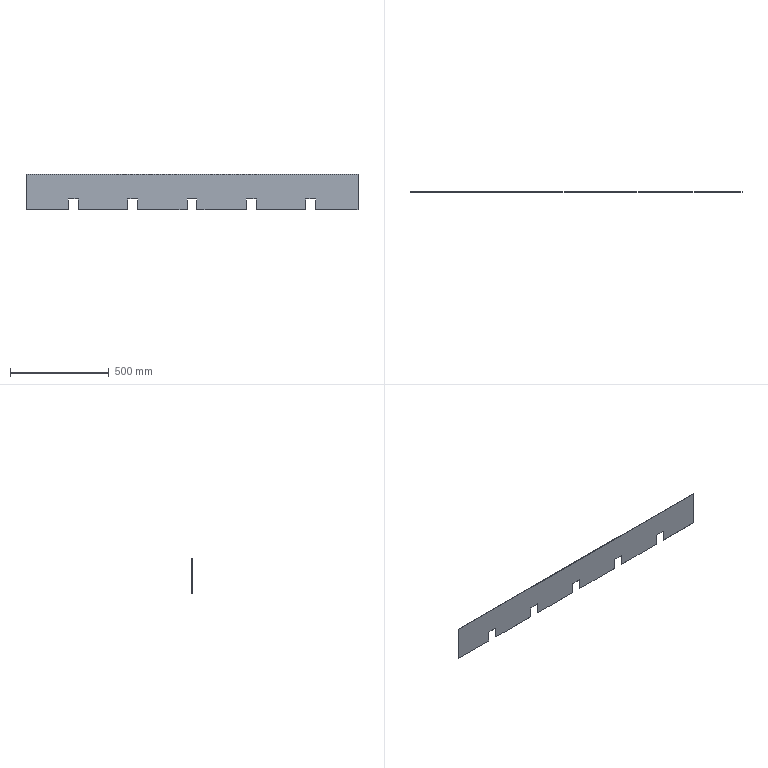Part | NX | features solid 2 | 1 solid | 26 faces | box 1680 x 2 x 180 mm | volume 577300 mm3 | plane 26
STEP:
#1=CARTESIAN_POINT('',(-575.,557.,-385.));
#2=VERTEX_POINT('',#1);
#3=CARTESIAN_POINT('',(-625.,557.,-385.));
#4=VERTEX_POINT('',#3);
#5=CARTESIAN_POINT('',(-770.,557.,-385.));
#6=DIRECTION('',(-1.,0.,0.));
#7=VECTOR('',#6,1000.);
#8=LINE('',#5,#7);
#9=EDGE_CURVE('',#2,#4,#8,.T.);
#10=ORIENTED_EDGE('',*,*,#9,.T.);
#11=CARTESIAN_POINT('',(-625.,557.,-440.));
#12=VERTEX_POINT('',#11);
#13=CARTESIAN_POINT('',(-625.,557.,-390.));
#14=DIRECTION('',(0.,0.,-1.));
#15=VECTOR('',#14,1000.);
#16=LINE('',#13,#15);
#17=EDGE_CURVE('',#4,#12,#16,.T.);
#18=ORIENTED_EDGE('',*,*,#17,.T.);
#19=CARTESIAN_POINT('',(-840.,557.,-440.));
#20=VERTEX_POINT('',#19);
#21=CARTESIAN_POINT('',(-770.,557.,-440.));
#22=DIRECTION('',(1.,0.,0.));
#23=VECTOR('',#22,1000.);
#24=LINE('',#21,#23);
#25=EDGE_CURVE('',#20,#12,#24,.T.);
#26=ORIENTED_EDGE('',*,*,#25,.F.);
#27=CARTESIAN_POINT('',(-840.,557.,-260.));
#28=VERTEX_POINT('',#27);
#29=CARTESIAN_POINT('',(-840.,557.,-390.));
#30=DIRECTION('',(0.,0.,-1.));
#31=VECTOR('',#30,1000.);
#32=LINE('',#29,#31);
#33=EDGE_CURVE('',#28,#20,#32,.T.);
#34=ORIENTED_EDGE('',*,*,#33,.F.);
#35=CARTESIAN_POINT('',(840.,557.,-260.));
#36=VERTEX_POINT('',#35);
#37=CARTESIAN_POINT('',(-900.,557.,-260.));
#38=DIRECTION('',(1.,0.,0.));
#39=VECTOR('',#38,1000.);
#40=LINE('',#37,#39);
#41=EDGE_CURVE('',#28,#36,#40,.T.);
#42=ORIENTED_EDGE('',*,*,#41,.T.);
#43=CARTESIAN_POINT('',(840.,557.,-440.));
#44=VERTEX_POINT('',#43);
#45=CARTESIAN_POINT('',(840.,557.,-390.));
#46=DIRECTION('',(0.,0.,-1.));
#47=VECTOR('',#46,1000.);
#48=LINE('',#45,#47);
#49=EDGE_CURVE('',#36,#44,#48,.T.);
#50=ORIENTED_EDGE('',*,*,#49,.T.);
#51=CARTESIAN_POINT('',(625.,557.,-440.));
#52=VERTEX_POINT('',#51);
#53=CARTESIAN_POINT('',(770.,557.,-440.));
#54=DIRECTION('',(-1.,0.,0.));
#55=VECTOR('',#54,1000.);
#56=LINE('',#53,#55);
#57=EDGE_CURVE('',#44,#52,#56,.T.);
#58=ORIENTED_EDGE('',*,*,#57,.T.);
#59=CARTESIAN_POINT('',(625.,557.,-385.));
#60=VERTEX_POINT('',#59);
#61=CARTESIAN_POINT('',(625.,557.,-390.));
#62=DIRECTION('',(0.,0.,-1.));
#63=VECTOR('',#62,1000.);
#64=LINE('',#61,#63);
#65=EDGE_CURVE('',#60,#52,#64,.T.);
#66=ORIENTED_EDGE('',*,*,#65,.F.);
#67=CARTESIAN_POINT('',(575.,557.,-385.));
#68=VERTEX_POINT('',#67);
#69=CARTESIAN_POINT('',(770.,557.,-385.));
#70=DIRECTION('',(1.,0.,0.));
#71=VECTOR('',#70,1000.);
#72=LINE('',#69,#71);
#73=EDGE_CURVE('',#68,#60,#72,.T.);
#74=ORIENTED_EDGE('',*,*,#73,.F.);
#75=CARTESIAN_POINT('',(575.,557.,-440.));
#76=VERTEX_POINT('',#75);
#77=CARTESIAN_POINT('',(575.,557.,-390.));
#78=DIRECTION('',(0.,0.,-1.));
#79=VECTOR('',#78,1000.);
#80=LINE('',#77,#79);
#81=EDGE_CURVE('',#68,#76,#80,.T.);
#82=ORIENTED_EDGE('',*,*,#81,.T.);
#83=CARTESIAN_POINT('',(325.,557.,-440.));
#84=VERTEX_POINT('',#83);
#85=CARTESIAN_POINT('',(770.,557.,-440.));
#86=DIRECTION('',(-1.,0.,0.));
#87=VECTOR('',#86,1000.);
#88=LINE('',#85,#87);
#89=EDGE_CURVE('',#76,#84,#88,.T.);
#90=ORIENTED_EDGE('',*,*,#89,.T.);
#91=CARTESIAN_POINT('',(325.,557.,-385.));
#92=VERTEX_POINT('',#91);
#93=CARTESIAN_POINT('',(325.,557.,-390.));
#94=DIRECTION('',(0.,0.,-1.));
#95=VECTOR('',#94,1000.);
#96=LINE('',#93,#95);
#97=EDGE_CURVE('',#92,#84,#96,.T.);
#98=ORIENTED_EDGE('',*,*,#97,.F.);
#99=CARTESIAN_POINT('',(275.,557.,-385.));
#100=VERTEX_POINT('',#99);
#101=CARTESIAN_POINT('',(770.,557.,-385.));
#102=DIRECTION('',(1.,0.,0.));
#103=VECTOR('',#102,1000.);
#104=LINE('',#101,#103);
#105=EDGE_CURVE('',#100,#92,#104,.T.);
#106=ORIENTED_EDGE('',*,*,#105,.F.);
#107=CARTESIAN_POINT('',(275.,557.,-440.));
#108=VERTEX_POINT('',#107);
#109=CARTESIAN_POINT('',(275.,557.,-390.));
#110=DIRECTION('',(0.,0.,-1.));
#111=VECTOR('',#110,1000.);
#112=LINE('',#109,#111);
#113=EDGE_CURVE('',#100,#108,#112,.T.);
#114=ORIENTED_EDGE('',*,*,#113,.T.);
#115=CARTESIAN_POINT('',(25.,557.,-440.));
#116=VERTEX_POINT('',#115);
#117=CARTESIAN_POINT('',(770.,557.,-440.));
#118=DIRECTION('',(-1.,0.,0.));
#119=VECTOR('',#118,1000.);
#120=LINE('',#117,#119);
#121=EDGE_CURVE('',#108,#116,#120,.T.);
#122=ORIENTED_EDGE('',*,*,#121,.T.);
#123=CARTESIAN_POINT('',(25.,557.,-385.));
#124=VERTEX_POINT('',#123);
#125=CARTESIAN_POINT('',(25.,557.,-390.));
#126=DIRECTION('',(0.,0.,-1.));
#127=VECTOR('',#126,1000.);
#128=LINE('',#125,#127);
#129=EDGE_CURVE('',#124,#116,#128,.T.);
#130=ORIENTED_EDGE('',*,*,#129,.F.);
#131=CARTESIAN_POINT('',(-25.,557.,-385.));
#132=VERTEX_POINT('',#131);
#133=CARTESIAN_POINT('',(-770.,557.,-385.));
#134=DIRECTION('',(1.,0.,0.));
#135=VECTOR('',#134,1000.);
#136=LINE('',#133,#135);
#137=EDGE_CURVE('',#132,#124,#136,.T.);
#138=ORIENTED_EDGE('',*,*,#137,.F.);
#139=CARTESIAN_POINT('',(-25.,557.,-440.));
#140=VERTEX_POINT('',#139);
#141=CARTESIAN_POINT('',(-25.,557.,-390.));
#142=DIRECTION('',(0.,0.,-1.));
#143=VECTOR('',#142,1000.);
#144=LINE('',#141,#143);
#145=EDGE_CURVE('',#132,#140,#144,.T.);
#146=ORIENTED_EDGE('',*,*,#145,.T.);
#147=CARTESIAN_POINT('',(-275.,557.,-440.));
#148=VERTEX_POINT('',#147);
#149=CARTESIAN_POINT('',(-770.,557.,-440.));
#150=DIRECTION('',(1.,0.,0.));
#151=VECTOR('',#150,1000.);
#152=LINE('',#149,#151);
#153=EDGE_CURVE('',#148,#140,#152,.T.);
#154=ORIENTED_EDGE('',*,*,#153,.F.);
#155=CARTESIAN_POINT('',(-275.,557.,-385.));
#156=VERTEX_POINT('',#155);
#157=CARTESIAN_POINT('',(-275.,557.,-390.));
#158=DIRECTION('',(0.,0.,-1.));
#159=VECTOR('',#158,1000.);
#160=LINE('',#157,#159);
#161=EDGE_CURVE('',#156,#148,#160,.T.);
#162=ORIENTED_EDGE('',*,*,#161,.F.);
#163=CARTESIAN_POINT('',(-325.,557.,-385.));
#164=VERTEX_POINT('',#163);
#165=CARTESIAN_POINT('',(-770.,557.,-385.));
#166=DIRECTION('',(-1.,0.,0.));
#167=VECTOR('',#166,1000.);
#168=LINE('',#165,#167);
#169=EDGE_CURVE('',#156,#164,#168,.T.);
#170=ORIENTED_EDGE('',*,*,#169,.T.);
#171=CARTESIAN_POINT('',(-325.,557.,-440.));
#172=VERTEX_POINT('',#171);
#173=CARTESIAN_POINT('',(-325.,557.,-390.));
#174=DIRECTION('',(0.,0.,-1.));
#175=VECTOR('',#174,1000.);
#176=LINE('',#173,#175);
#177=EDGE_CURVE('',#164,#172,#176,.T.);
#178=ORIENTED_EDGE('',*,*,#177,.T.);
#179=CARTESIAN_POINT('',(-575.,557.,-440.));
#180=VERTEX_POINT('',#179);
#181=CARTESIAN_POINT('',(-770.,557.,-440.));
#182=DIRECTION('',(1.,0.,0.));
#183=VECTOR('',#182,1000.);
#184=LINE('',#181,#183);
#185=EDGE_CURVE('',#180,#172,#184,.T.);
#186=ORIENTED_EDGE('',*,*,#185,.F.);
#187=CARTESIAN_POINT('',(-575.,557.,-390.));
#188=DIRECTION('',(0.,0.,-1.));
#189=VECTOR('',#188,1000.);
#190=LINE('',#187,#189);
#191=EDGE_CURVE('',#2,#180,#190,.T.);
#192=ORIENTED_EDGE('',*,*,#191,.F.);
#193=EDGE_LOOP('',(#10,#18,#26,#34,#42,#50,#58,#66,#74,#82,#90,#98,#106,#114,#122,#130,#138,#146,#154,#162,#170,#178,#186,#192));
#194=FACE_BOUND('',#193,.T.);
#195=CARTESIAN_POINT('',(-770.,557.,-390.));
#196=DIRECTION('',(0.,1.,0.));
#197=DIRECTION('',(0.,0.,1.));
#198=AXIS2_PLACEMENT_3D('',#195,#196,#197);
#199=PLANE('',#198);
#200=ADVANCED_FACE('',(#194),#199,.T.);
#201=CARTESIAN_POINT('',(-575.,555.,-385.));
#202=VERTEX_POINT('',#201);
#203=CARTESIAN_POINT('',(-575.,555.,-440.));
#204=VERTEX_POINT('',#203);
#205=CARTESIAN_POINT('',(-575.,555.,-390.));
#206=DIRECTION('',(0.,0.,-1.));
#207=VECTOR('',#206,1000.);
#208=LINE('',#205,#207);
#209=EDGE_CURVE('',#202,#204,#208,.T.);
#210=ORIENTED_EDGE('',*,*,#209,.T.);
#211=CARTESIAN_POINT('',(-325.,555.,-440.));
#212=VERTEX_POINT('',#211);
#213=CARTESIAN_POINT('',(-770.,555.,-440.));
#214=DIRECTION('',(1.,0.,0.));
#215=VECTOR('',#214,1000.);
#216=LINE('',#213,#215);
#217=EDGE_CURVE('',#204,#212,#216,.T.);
#218=ORIENTED_EDGE('',*,*,#217,.T.);
#219=CARTESIAN_POINT('',(-325.,555.,-385.));
#220=VERTEX_POINT('',#219);
#221=CARTESIAN_POINT('',(-325.,555.,-390.));
#222=DIRECTION('',(0.,0.,-1.));
#223=VECTOR('',#222,1000.);
#224=LINE('',#221,#223);
#225=EDGE_CURVE('',#220,#212,#224,.T.);
#226=ORIENTED_EDGE('',*,*,#225,.F.);
#227=CARTESIAN_POINT('',(-275.,555.,-385.));
#228=VERTEX_POINT('',#227);
#229=CARTESIAN_POINT('',(-770.,555.,-385.));
#230=DIRECTION('',(-1.,0.,0.));
#231=VECTOR('',#230,1000.);
#232=LINE('',#229,#231);
#233=EDGE_CURVE('',#228,#220,#232,.T.);
#234=ORIENTED_EDGE('',*,*,#233,.F.);
#235=CARTESIAN_POINT('',(-275.,555.,-440.));
#236=VERTEX_POINT('',#235);
#237=CARTESIAN_POINT('',(-275.,555.,-390.));
#238=DIRECTION('',(0.,0.,-1.));
#239=VECTOR('',#238,1000.);
#240=LINE('',#237,#239);
#241=EDGE_CURVE('',#228,#236,#240,.T.);
#242=ORIENTED_EDGE('',*,*,#241,.T.);
#243=CARTESIAN_POINT('',(-25.,555.,-440.));
#244=VERTEX_POINT('',#243);
#245=CARTESIAN_POINT('',(-770.,555.,-440.));
#246=DIRECTION('',(1.,0.,0.));
#247=VECTOR('',#246,1000.);
#248=LINE('',#245,#247);
#249=EDGE_CURVE('',#236,#244,#248,.T.);
#250=ORIENTED_EDGE('',*,*,#249,.T.);
#251=CARTESIAN_POINT('',(-25.,555.,-385.));
#252=VERTEX_POINT('',#251);
#253=CARTESIAN_POINT('',(-25.,555.,-390.));
#254=DIRECTION('',(0.,0.,-1.));
#255=VECTOR('',#254,1000.);
#256=LINE('',#253,#255);
#257=EDGE_CURVE('',#252,#244,#256,.T.);
#258=ORIENTED_EDGE('',*,*,#257,.F.);
#259=CARTESIAN_POINT('',(25.,555.,-385.));
#260=VERTEX_POINT('',#259);
#261=CARTESIAN_POINT('',(-770.,555.,-385.));
#262=DIRECTION('',(1.,0.,0.));
#263=VECTOR('',#262,1000.);
#264=LINE('',#261,#263);
#265=EDGE_CURVE('',#252,#260,#264,.T.);
#266=ORIENTED_EDGE('',*,*,#265,.T.);
#267=CARTESIAN_POINT('',(25.,555.,-440.));
#268=VERTEX_POINT('',#267);
#269=CARTESIAN_POINT('',(25.,555.,-390.));
#270=DIRECTION('',(0.,0.,-1.));
#271=VECTOR('',#270,1000.);
#272=LINE('',#269,#271);
#273=EDGE_CURVE('',#260,#268,#272,.T.);
#274=ORIENTED_EDGE('',*,*,#273,.T.);
#275=CARTESIAN_POINT('',(275.,555.,-440.));
#276=VERTEX_POINT('',#275);
#277=CARTESIAN_POINT('',(770.,555.,-440.));
#278=DIRECTION('',(-1.,0.,0.));
#279=VECTOR('',#278,1000.);
#280=LINE('',#277,#279);
#281=EDGE_CURVE('',#276,#268,#280,.T.);
#282=ORIENTED_EDGE('',*,*,#281,.F.);
#283=CARTESIAN_POINT('',(275.,555.,-385.));
#284=VERTEX_POINT('',#283);
#285=CARTESIAN_POINT('',(275.,555.,-390.));
#286=DIRECTION('',(0.,0.,-1.));
#287=VECTOR('',#286,1000.);
#288=LINE('',#285,#287);
#289=EDGE_CURVE('',#284,#276,#288,.T.);
#290=ORIENTED_EDGE('',*,*,#289,.F.);
#291=CARTESIAN_POINT('',(325.,555.,-385.));
#292=VERTEX_POINT('',#291);
#293=CARTESIAN_POINT('',(770.,555.,-385.));
#294=DIRECTION('',(1.,0.,0.));
#295=VECTOR('',#294,1000.);
#296=LINE('',#293,#295);
#297=EDGE_CURVE('',#284,#292,#296,.T.);
#298=ORIENTED_EDGE('',*,*,#297,.T.);
#299=CARTESIAN_POINT('',(325.,555.,-440.));
#300=VERTEX_POINT('',#299);
#301=CARTESIAN_POINT('',(325.,555.,-390.));
#302=DIRECTION('',(0.,0.,-1.));
#303=VECTOR('',#302,1000.);
#304=LINE('',#301,#303);
#305=EDGE_CURVE('',#292,#300,#304,.T.);
#306=ORIENTED_EDGE('',*,*,#305,.T.);
#307=CARTESIAN_POINT('',(575.,555.,-440.));
#308=VERTEX_POINT('',#307);
#309=CARTESIAN_POINT('',(770.,555.,-440.));
#310=DIRECTION('',(-1.,0.,0.));
#311=VECTOR('',#310,1000.);
#312=LINE('',#309,#311);
#313=EDGE_CURVE('',#308,#300,#312,.T.);
#314=ORIENTED_EDGE('',*,*,#313,.F.);
#315=CARTESIAN_POINT('',(575.,555.,-385.));
#316=VERTEX_POINT('',#315);
#317=CARTESIAN_POINT('',(575.,555.,-390.));
#318=DIRECTION('',(0.,0.,-1.));
#319=VECTOR('',#318,1000.);
#320=LINE('',#317,#319);
#321=EDGE_CURVE('',#316,#308,#320,.T.);
#322=ORIENTED_EDGE('',*,*,#321,.F.);
#323=CARTESIAN_POINT('',(625.,555.,-385.));
#324=VERTEX_POINT('',#323);
#325=CARTESIAN_POINT('',(770.,555.,-385.));
#326=DIRECTION('',(1.,0.,0.));
#327=VECTOR('',#326,1000.);
#328=LINE('',#325,#327);
#329=EDGE_CURVE('',#316,#324,#328,.T.);
#330=ORIENTED_EDGE('',*,*,#329,.T.);
#331=CARTESIAN_POINT('',(625.,555.,-440.));
#332=VERTEX_POINT('',#331);
#333=CARTESIAN_POINT('',(625.,555.,-390.));
#334=DIRECTION('',(0.,0.,-1.));
#335=VECTOR('',#334,1000.);
#336=LINE('',#333,#335);
#337=EDGE_CURVE('',#324,#332,#336,.T.);
#338=ORIENTED_EDGE('',*,*,#337,.T.);
#339=CARTESIAN_POINT('',(840.,555.,-440.));
#340=VERTEX_POINT('',#339);
#341=CARTESIAN_POINT('',(770.,555.,-440.));
#342=DIRECTION('',(-1.,0.,0.));
#343=VECTOR('',#342,1000.);
#344=LINE('',#341,#343);
#345=EDGE_CURVE('',#340,#332,#344,.T.);
#346=ORIENTED_EDGE('',*,*,#345,.F.);
#347=CARTESIAN_POINT('',(840.,555.,-260.));
#348=VERTEX_POINT('',#347);
#349=CARTESIAN_POINT('',(840.,555.,-390.));
#350=DIRECTION('',(0.,0.,-1.));
#351=VECTOR('',#350,1000.);
#352=LINE('',#349,#351);
#353=EDGE_CURVE('',#348,#340,#352,.T.);
#354=ORIENTED_EDGE('',*,*,#353,.F.);
#355=CARTESIAN_POINT('',(-840.,555.,-260.));
#356=VERTEX_POINT('',#355);
#357=CARTESIAN_POINT('',(-900.,555.,-260.));
#358=DIRECTION('',(1.,0.,0.));
#359=VECTOR('',#358,1000.);
#360=LINE('',#357,#359);
#361=EDGE_CURVE('',#356,#348,#360,.T.);
#362=ORIENTED_EDGE('',*,*,#361,.F.);
#363=CARTESIAN_POINT('',(-840.,555.,-440.));
#364=VERTEX_POINT('',#363);
#365=CARTESIAN_POINT('',(-840.,555.,-390.));
#366=DIRECTION('',(0.,0.,-1.));
#367=VECTOR('',#366,1000.);
#368=LINE('',#365,#367);
#369=EDGE_CURVE('',#356,#364,#368,.T.);
#370=ORIENTED_EDGE('',*,*,#369,.T.);
#371=CARTESIAN_POINT('',(-625.,555.,-440.));
#372=VERTEX_POINT('',#371);
#373=CARTESIAN_POINT('',(-770.,555.,-440.));
#374=DIRECTION('',(1.,0.,0.));
#375=VECTOR('',#374,1000.);
#376=LINE('',#373,#375);
#377=EDGE_CURVE('',#364,#372,#376,.T.);
#378=ORIENTED_EDGE('',*,*,#377,.T.);
#379=CARTESIAN_POINT('',(-625.,555.,-385.));
#380=VERTEX_POINT('',#379);
#381=CARTESIAN_POINT('',(-625.,555.,-390.));
#382=DIRECTION('',(0.,0.,-1.));
#383=VECTOR('',#382,1000.);
#384=LINE('',#381,#383);
#385=EDGE_CURVE('',#380,#372,#384,.T.);
#386=ORIENTED_EDGE('',*,*,#385,.F.);
#387=CARTESIAN_POINT('',(-770.,555.,-385.));
#388=DIRECTION('',(-1.,0.,0.));
#389=VECTOR('',#388,1000.);
#390=LINE('',#387,#389);
#391=EDGE_CURVE('',#202,#380,#390,.T.);
#392=ORIENTED_EDGE('',*,*,#391,.F.);
#393=EDGE_LOOP('',(#210,#218,#226,#234,#242,#250,#258,#266,#274,#282,#290,#298,#306,#314,#322,#330,#338,#346,#354,#362,#370,#378,#386,#392));
#394=FACE_BOUND('',#393,.T.);
#395=CARTESIAN_POINT('',(-770.,555.,-390.));
#396=DIRECTION('',(0.,1.,0.));
#397=DIRECTION('',(0.,0.,1.));
#398=AXIS2_PLACEMENT_3D('',#395,#396,#397);
#399=PLANE('',#398);
#400=ADVANCED_FACE('',(#394),#399,.F.);
#401=ORIENTED_EDGE('',*,*,#185,.T.);
#402=CARTESIAN_POINT('',(-325.,555.,-440.));
#403=DIRECTION('',(0.,-1.,0.));
#404=VECTOR('',#403,1000.);
#405=LINE('',#402,#404);
#406=EDGE_CURVE('',#172,#212,#405,.T.);
#407=ORIENTED_EDGE('',*,*,#406,.T.);
#408=ORIENTED_EDGE('',*,*,#217,.F.);
#409=CARTESIAN_POINT('',(-575.,555.,-440.));
#410=DIRECTION('',(0.,-1.,0.));
#411=VECTOR('',#410,1000.);
#412=LINE('',#409,#411);
#413=EDGE_CURVE('',#180,#204,#412,.T.);
#414=ORIENTED_EDGE('',*,*,#413,.F.);
#415=EDGE_LOOP('',(#401,#407,#408,#414));
#416=FACE_BOUND('',#415,.T.);
#417=CARTESIAN_POINT('',(-770.,555.,-440.));
#418=DIRECTION('',(0.,0.,-1.));
#419=DIRECTION('',(-1.,0.,0.));
#420=AXIS2_PLACEMENT_3D('',#417,#418,#419);
#421=PLANE('',#420);
#422=ADVANCED_FACE('',(#416),#421,.T.);
#423=CARTESIAN_POINT('',(-25.,555.,-440.));
#424=DIRECTION('',(0.,-1.,0.));
#425=VECTOR('',#424,1000.);
#426=LINE('',#423,#425);
#427=EDGE_CURVE('',#140,#244,#426,.T.);
#428=ORIENTED_EDGE('',*,*,#427,.T.);
#429=ORIENTED_EDGE('',*,*,#249,.F.);
#430=CARTESIAN_POINT('',(-275.,555.,-440.));
#431=DIRECTION('',(0.,-1.,0.));
#432=VECTOR('',#431,1000.);
#433=LINE('',#430,#432);
#434=EDGE_CURVE('',#148,#236,#433,.T.);
#435=ORIENTED_EDGE('',*,*,#434,.F.);
#436=ORIENTED_EDGE('',*,*,#153,.T.);
#437=EDGE_LOOP('',(#428,#429,#435,#436));
#438=FACE_BOUND('',#437,.T.);
#439=CARTESIAN_POINT('',(-770.,555.,-440.));
#440=DIRECTION('',(0.,0.,-1.));
#441=DIRECTION('',(-1.,0.,0.));
#442=AXIS2_PLACEMENT_3D('',#439,#440,#441);
#443=PLANE('',#442);
#444=ADVANCED_FACE('',(#438),#443,.T.);
#445=CARTESIAN_POINT('',(-625.,555.,-440.));
#446=DIRECTION('',(0.,-1.,0.));
#447=VECTOR('',#446,1000.);
#448=LINE('',#445,#447);
#449=EDGE_CURVE('',#12,#372,#448,.T.);
#450=ORIENTED_EDGE('',*,*,#449,.T.);
#451=ORIENTED_EDGE('',*,*,#377,.F.);
#452=CARTESIAN_POINT('',(-840.,555.,-440.));
#453=DIRECTION('',(0.,1.,0.));
#454=VECTOR('',#453,1000.);
#455=LINE('',#452,#454);
#456=EDGE_CURVE('',#364,#20,#455,.T.);
#457=ORIENTED_EDGE('',*,*,#456,.T.);
#458=ORIENTED_EDGE('',*,*,#25,.T.);
#459=EDGE_LOOP('',(#450,#451,#457,#458));
#460=FACE_BOUND('',#459,.T.);
#461=CARTESIAN_POINT('',(-770.,555.,-440.));
#462=DIRECTION('',(0.,0.,-1.));
#463=DIRECTION('',(-1.,0.,0.));
#464=AXIS2_PLACEMENT_3D('',#461,#462,#463);
#465=PLANE('',#464);
#466=ADVANCED_FACE('',(#460),#465,.T.);
#467=ORIENTED_EDGE('',*,*,#41,.F.);
#468=CARTESIAN_POINT('',(-840.,375.,-260.));
#469=DIRECTION('',(0.,1.,0.));
#470=VECTOR('',#469,1000.);
#471=LINE('',#468,#470);
#472=EDGE_CURVE('',#356,#28,#471,.T.);
#473=ORIENTED_EDGE('',*,*,#472,.F.);
#474=ORIENTED_EDGE('',*,*,#361,.T.);
#475=CARTESIAN_POINT('',(840.,375.,-260.));
#476=DIRECTION('',(0.,1.,0.));
#477=VECTOR('',#476,1000.);
#478=LINE('',#475,#477);
#479=EDGE_CURVE('',#348,#36,#478,.T.);
#480=ORIENTED_EDGE('',*,*,#479,.T.);
#481=EDGE_LOOP('',(#467,#473,#474,#480));
#482=FACE_BOUND('',#481,.T.);
#483=CARTESIAN_POINT('',(-900.,375.,-260.));
#484=DIRECTION('',(0.,0.,-1.));
#485=DIRECTION('',(1.,0.,0.));
#486=AXIS2_PLACEMENT_3D('',#483,#484,#485);
#487=PLANE('',#486);
#488=ADVANCED_FACE('',(#482),#487,.F.);
#489=ORIENTED_EDGE('',*,*,#472,.T.);
#490=ORIENTED_EDGE('',*,*,#33,.T.);
#491=ORIENTED_EDGE('',*,*,#456,.F.);
#492=ORIENTED_EDGE('',*,*,#369,.F.);
#493=EDGE_LOOP('',(#489,#490,#491,#492));
#494=FACE_BOUND('',#493,.T.);
#495=CARTESIAN_POINT('',(-840.,555.,-390.));
#496=DIRECTION('',(-1.,0.,0.));
#497=DIRECTION('',(0.,0.,1.));
#498=AXIS2_PLACEMENT_3D('',#495,#496,#497);
#499=PLANE('',#498);
#500=ADVANCED_FACE('',(#494),#499,.T.);
#501=ORIENTED_EDGE('',*,*,#169,.F.);
#502=CARTESIAN_POINT('',(-275.,650.,-385.));
#503=DIRECTION('',(0.,-1.,0.));
#504=VECTOR('',#503,1000.);
#505=LINE('',#502,#504);
#506=EDGE_CURVE('',#156,#228,#505,.T.);
#507=ORIENTED_EDGE('',*,*,#506,.T.);
#508=ORIENTED_EDGE('',*,*,#233,.T.);
#509=CARTESIAN_POINT('',(-325.,650.,-385.));
#510=DIRECTION('',(0.,-1.,0.));
#511=VECTOR('',#510,1000.);
#512=LINE('',#509,#511);
#513=EDGE_CURVE('',#164,#220,#512,.T.);
#514=ORIENTED_EDGE('',*,*,#513,.F.);
#515=EDGE_LOOP('',(#501,#507,#508,#514));
#516=FACE_BOUND('',#515,.T.);
#517=CARTESIAN_POINT('',(-320.,650.,-385.));
#518=DIRECTION('',(0.,0.,1.));
#519=DIRECTION('',(-1.,0.,0.));
#520=AXIS2_PLACEMENT_3D('',#517,#518,#519);
#521=PLANE('',#520);
#522=ADVANCED_FACE('',(#516),#521,.F.);
#523=ORIENTED_EDGE('',*,*,#506,.F.);
#524=ORIENTED_EDGE('',*,*,#161,.T.);
#525=ORIENTED_EDGE('',*,*,#434,.T.);
#526=ORIENTED_EDGE('',*,*,#241,.F.);
#527=EDGE_LOOP('',(#523,#524,#525,#526));
#528=FACE_BOUND('',#527,.T.);
#529=CARTESIAN_POINT('',(-275.,650.,-560.));
#530=DIRECTION('',(-1.,0.,0.));
#531=DIRECTION('',(0.,0.,-1.));
#532=AXIS2_PLACEMENT_3D('',#529,#530,#531);
#533=PLANE('',#532);
#534=ADVANCED_FACE('',(#528),#533,.T.);
#535=ORIENTED_EDGE('',*,*,#177,.F.);
#536=ORIENTED_EDGE('',*,*,#513,.T.);
#537=ORIENTED_EDGE('',*,*,#225,.T.);
#538=ORIENTED_EDGE('',*,*,#406,.F.);
#539=EDGE_LOOP('',(#535,#536,#537,#538));
#540=FACE_BOUND('',#539,.T.);
#541=CARTESIAN_POINT('',(-325.,650.,-560.));
#542=DIRECTION('',(-1.,0.,0.));
#543=DIRECTION('',(0.,0.,-1.));
#544=AXIS2_PLACEMENT_3D('',#541,#542,#543);
#545=PLANE('',#544);
#546=ADVANCED_FACE('',(#540),#545,.F.);
#547=CARTESIAN_POINT('',(-25.,650.,-385.));
#548=DIRECTION('',(0.,-1.,0.));
#549=VECTOR('',#548,1000.);
#550=LINE('',#547,#549);
#551=EDGE_CURVE('',#132,#252,#550,.T.);
#552=ORIENTED_EDGE('',*,*,#551,.F.);
#553=ORIENTED_EDGE('',*,*,#137,.T.);
#554=CARTESIAN_POINT('',(25.,650.,-385.));
#555=DIRECTION('',(0.,-1.,0.));
#556=VECTOR('',#555,1000.);
#557=LINE('',#554,#556);
#558=EDGE_CURVE('',#124,#260,#557,.T.);
#559=ORIENTED_EDGE('',*,*,#558,.T.);
#560=ORIENTED_EDGE('',*,*,#265,.F.);
#561=EDGE_LOOP('',(#552,#553,#559,#560));
#562=FACE_BOUND('',#561,.T.);
#563=CARTESIAN_POINT('',(20.,650.,-385.));
#564=DIRECTION('',(0.,0.,-1.));
#565=DIRECTION('',(1.,0.,0.));
#566=AXIS2_PLACEMENT_3D('',#563,#564,#565);
#567=PLANE('',#566);
#568=ADVANCED_FACE('',(#562),#567,.T.);
#569=ORIENTED_EDGE('',*,*,#145,.F.);
#570=ORIENTED_EDGE('',*,*,#551,.T.);
#571=ORIENTED_EDGE('',*,*,#257,.T.);
#572=ORIENTED_EDGE('',*,*,#427,.F.);
#573=EDGE_LOOP('',(#569,#570,#571,#572));
#574=FACE_BOUND('',#573,.T.);
#575=CARTESIAN_POINT('',(-25.,650.,-540.));
#576=DIRECTION('',(-1.,0.,0.));
#577=DIRECTION('',(0.,0.,-1.));
#578=AXIS2_PLACEMENT_3D('',#575,#576,#577);
#579=PLANE('',#578);
#580=ADVANCED_FACE('',(#574),#579,.F.);
#581=ORIENTED_EDGE('',*,*,#9,.F.);
#582=CARTESIAN_POINT('',(-575.,650.,-385.));
#583=DIRECTION('',(0.,-1.,0.));
#584=VECTOR('',#583,1000.);
#585=LINE('',#582,#584);
#586=EDGE_CURVE('',#2,#202,#585,.T.);
#587=ORIENTED_EDGE('',*,*,#586,.T.);
#588=ORIENTED_EDGE('',*,*,#391,.T.);
#589=CARTESIAN_POINT('',(-625.,650.,-385.));
#590=DIRECTION('',(0.,-1.,0.));
#591=VECTOR('',#590,1000.);
#592=LINE('',#589,#591);
#593=EDGE_CURVE('',#4,#380,#592,.T.);
#594=ORIENTED_EDGE('',*,*,#593,.F.);
#595=EDGE_LOOP('',(#581,#587,#588,#594));
#596=FACE_BOUND('',#595,.T.);
#597=CARTESIAN_POINT('',(-620.,650.,-385.));
#598=DIRECTION('',(0.,0.,1.));
#599=DIRECTION('',(-1.,0.,0.));
#600=AXIS2_PLACEMENT_3D('',#597,#598,#599);
#601=PLANE('',#600);
#602=ADVANCED_FACE('',(#596),#601,.F.);
#603=ORIENTED_EDGE('',*,*,#586,.F.);
#604=ORIENTED_EDGE('',*,*,#191,.T.);
#605=ORIENTED_EDGE('',*,*,#413,.T.);
#606=ORIENTED_EDGE('',*,*,#209,.F.);
#607=EDGE_LOOP('',(#603,#604,#605,#606));
#608=FACE_BOUND('',#607,.T.);
#609=CARTESIAN_POINT('',(-575.,650.,-560.));
#610=DIRECTION('',(-1.,0.,0.));
#611=DIRECTION('',(0.,0.,-1.));
#612=AXIS2_PLACEMENT_3D('',#609,#610,#611);
#613=PLANE('',#612);
#614=ADVANCED_FACE('',(#608),#613,.T.);
#615=ORIENTED_EDGE('',*,*,#17,.F.);
#616=ORIENTED_EDGE('',*,*,#593,.T.);
#617=ORIENTED_EDGE('',*,*,#385,.T.);
#618=ORIENTED_EDGE('',*,*,#449,.F.);
#619=EDGE_LOOP('',(#615,#616,#617,#618));
#620=FACE_BOUND('',#619,.T.);
#621=CARTESIAN_POINT('',(-625.,650.,-560.));
#622=DIRECTION('',(-1.,0.,0.));
#623=DIRECTION('',(0.,0.,-1.));
#624=AXIS2_PLACEMENT_3D('',#621,#622,#623);
#625=PLANE('',#624);
#626=ADVANCED_FACE('',(#620),#625,.F.);
#627=ORIENTED_EDGE('',*,*,#89,.F.);
#628=CARTESIAN_POINT('',(575.,555.,-440.));
#629=DIRECTION('',(0.,-1.,0.));
#630=VECTOR('',#629,1000.);
#631=LINE('',#628,#630);
#632=EDGE_CURVE('',#76,#308,#631,.T.);
#633=ORIENTED_EDGE('',*,*,#632,.T.);
#634=ORIENTED_EDGE('',*,*,#313,.T.);
#635=CARTESIAN_POINT('',(325.,555.,-440.));
#636=DIRECTION('',(0.,-1.,0.));
#637=VECTOR('',#636,1000.);
#638=LINE('',#635,#637);
#639=EDGE_CURVE('',#84,#300,#638,.T.);
#640=ORIENTED_EDGE('',*,*,#639,.F.);
#641=EDGE_LOOP('',(#627,#633,#634,#640));
#642=FACE_BOUND('',#641,.T.);
#643=CARTESIAN_POINT('',(770.,555.,-440.));
#644=DIRECTION('',(0.,0.,-1.));
#645=DIRECTION('',(1.,0.,0.));
#646=AXIS2_PLACEMENT_3D('',#643,#644,#645);
#647=PLANE('',#646);
#648=ADVANCED_FACE('',(#642),#647,.T.);
#649=CARTESIAN_POINT('',(25.,555.,-440.));
#650=DIRECTION('',(0.,-1.,0.));
#651=VECTOR('',#650,1000.);
#652=LINE('',#649,#651);
#653=EDGE_CURVE('',#116,#268,#652,.T.);
#654=ORIENTED_EDGE('',*,*,#653,.F.);
#655=ORIENTED_EDGE('',*,*,#121,.F.);
#656=CARTESIAN_POINT('',(275.,555.,-440.));
#657=DIRECTION('',(0.,-1.,0.));
#658=VECTOR('',#657,1000.);
#659=LINE('',#656,#658);
#660=EDGE_CURVE('',#108,#276,#659,.T.);
#661=ORIENTED_EDGE('',*,*,#660,.T.);
#662=ORIENTED_EDGE('',*,*,#281,.T.);
#663=EDGE_LOOP('',(#654,#655,#661,#662));
#664=FACE_BOUND('',#663,.T.);
#665=CARTESIAN_POINT('',(770.,555.,-440.));
#666=DIRECTION('',(0.,0.,-1.));
#667=DIRECTION('',(1.,0.,0.));
#668=AXIS2_PLACEMENT_3D('',#665,#666,#667);
#669=PLANE('',#668);
#670=ADVANCED_FACE('',(#664),#669,.T.);
#671=CARTESIAN_POINT('',(625.,555.,-440.));
#672=DIRECTION('',(0.,-1.,0.));
#673=VECTOR('',#672,1000.);
#674=LINE('',#671,#673);
#675=EDGE_CURVE('',#52,#332,#674,.T.);
#676=ORIENTED_EDGE('',*,*,#675,.F.);
#677=ORIENTED_EDGE('',*,*,#57,.F.);
#678=CARTESIAN_POINT('',(840.,555.,-440.));
#679=DIRECTION('',(0.,1.,0.));
#680=VECTOR('',#679,1000.);
#681=LINE('',#678,#680);
#682=EDGE_CURVE('',#340,#44,#681,.T.);
#683=ORIENTED_EDGE('',*,*,#682,.F.);
#684=ORIENTED_EDGE('',*,*,#345,.T.);
#685=EDGE_LOOP('',(#676,#677,#683,#684));
#686=FACE_BOUND('',#685,.T.);
#687=CARTESIAN_POINT('',(770.,555.,-440.));
#688=DIRECTION('',(0.,0.,-1.));
#689=DIRECTION('',(1.,0.,0.));
#690=AXIS2_PLACEMENT_3D('',#687,#688,#689);
#691=PLANE('',#690);
#692=ADVANCED_FACE('',(#686),#691,.T.);
#693=ORIENTED_EDGE('',*,*,#479,.F.);
#694=ORIENTED_EDGE('',*,*,#353,.T.);
#695=ORIENTED_EDGE('',*,*,#682,.T.);
#696=ORIENTED_EDGE('',*,*,#49,.F.);
#697=EDGE_LOOP('',(#693,#694,#695,#696));
#698=FACE_BOUND('',#697,.T.);
#699=CARTESIAN_POINT('',(840.,555.,-390.));
#700=DIRECTION('',(1.,0.,0.));
#701=DIRECTION('',(0.,0.,1.));
#702=AXIS2_PLACEMENT_3D('',#699,#700,#701);
#703=PLANE('',#702);
#704=ADVANCED_FACE('',(#698),#703,.T.);
#705=ORIENTED_EDGE('',*,*,#105,.T.);
#706=CARTESIAN_POINT('',(325.,650.,-385.));
#707=DIRECTION('',(0.,-1.,0.));
#708=VECTOR('',#707,1000.);
#709=LINE('',#706,#708);
#710=EDGE_CURVE('',#92,#292,#709,.T.);
#711=ORIENTED_EDGE('',*,*,#710,.T.);
#712=ORIENTED_EDGE('',*,*,#297,.F.);
#713=CARTESIAN_POINT('',(275.,650.,-385.));
#714=DIRECTION('',(0.,-1.,0.));
#715=VECTOR('',#714,1000.);
#716=LINE('',#713,#715);
#717=EDGE_CURVE('',#100,#284,#716,.T.);
#718=ORIENTED_EDGE('',*,*,#717,.F.);
#719=EDGE_LOOP('',(#705,#711,#712,#718));
#720=FACE_BOUND('',#719,.T.);
#721=CARTESIAN_POINT('',(320.,650.,-385.));
#722=DIRECTION('',(0.,0.,1.));
#723=DIRECTION('',(1.,0.,0.));
#724=AXIS2_PLACEMENT_3D('',#721,#722,#723);
#725=PLANE('',#724);
#726=ADVANCED_FACE('',(#720),#725,.F.);
#727=ORIENTED_EDGE('',*,*,#717,.T.);
#728=ORIENTED_EDGE('',*,*,#289,.T.);
#729=ORIENTED_EDGE('',*,*,#660,.F.);
#730=ORIENTED_EDGE('',*,*,#113,.F.);
#731=EDGE_LOOP('',(#727,#728,#729,#730));
#732=FACE_BOUND('',#731,.T.);
#733=CARTESIAN_POINT('',(275.,650.,-560.));
#734=DIRECTION('',(1.,0.,0.));
#735=DIRECTION('',(0.,0.,-1.));
#736=AXIS2_PLACEMENT_3D('',#733,#734,#735);
#737=PLANE('',#736);
#738=ADVANCED_FACE('',(#732),#737,.T.);
#739=ORIENTED_EDGE('',*,*,#97,.T.);
#740=ORIENTED_EDGE('',*,*,#639,.T.);
#741=ORIENTED_EDGE('',*,*,#305,.F.);
#742=ORIENTED_EDGE('',*,*,#710,.F.);
#743=EDGE_LOOP('',(#739,#740,#741,#742));
#744=FACE_BOUND('',#743,.T.);
#745=CARTESIAN_POINT('',(325.,650.,-560.));
#746=DIRECTION('',(1.,0.,0.));
#747=DIRECTION('',(0.,0.,-1.));
#748=AXIS2_PLACEMENT_3D('',#745,#746,#747);
#749=PLANE('',#748);
#750=ADVANCED_FACE('',(#744),#749,.F.);
#751=ORIENTED_EDGE('',*,*,#129,.T.);
#752=ORIENTED_EDGE('',*,*,#653,.T.);
#753=ORIENTED_EDGE('',*,*,#273,.F.);
#754=ORIENTED_EDGE('',*,*,#558,.F.);
#755=EDGE_LOOP('',(#751,#752,#753,#754));
#756=FACE_BOUND('',#755,.T.);
#757=CARTESIAN_POINT('',(25.,650.,-540.));
#758=DIRECTION('',(1.,0.,0.));
#759=DIRECTION('',(0.,0.,-1.));
#760=AXIS2_PLACEMENT_3D('',#757,#758,#759);
#761=PLANE('',#760);
#762=ADVANCED_FACE('',(#756),#761,.F.);
#763=ORIENTED_EDGE('',*,*,#73,.T.);
#764=CARTESIAN_POINT('',(625.,650.,-385.));
#765=DIRECTION('',(0.,-1.,0.));
#766=VECTOR('',#765,1000.);
#767=LINE('',#764,#766);
#768=EDGE_CURVE('',#60,#324,#767,.T.);
#769=ORIENTED_EDGE('',*,*,#768,.T.);
#770=ORIENTED_EDGE('',*,*,#329,.F.);
#771=CARTESIAN_POINT('',(575.,650.,-385.));
#772=DIRECTION('',(0.,-1.,0.));
#773=VECTOR('',#772,1000.);
#774=LINE('',#771,#773);
#775=EDGE_CURVE('',#68,#316,#774,.T.);
#776=ORIENTED_EDGE('',*,*,#775,.F.);
#777=EDGE_LOOP('',(#763,#769,#770,#776));
#778=FACE_BOUND('',#777,.T.);
#779=CARTESIAN_POINT('',(620.,650.,-385.));
#780=DIRECTION('',(0.,0.,1.));
#781=DIRECTION('',(1.,0.,0.));
#782=AXIS2_PLACEMENT_3D('',#779,#780,#781);
#783=PLANE('',#782);
#784=ADVANCED_FACE('',(#778),#783,.F.);
#785=ORIENTED_EDGE('',*,*,#775,.T.);
#786=ORIENTED_EDGE('',*,*,#321,.T.);
#787=ORIENTED_EDGE('',*,*,#632,.F.);
#788=ORIENTED_EDGE('',*,*,#81,.F.);
#789=EDGE_LOOP('',(#785,#786,#787,#788));
#790=FACE_BOUND('',#789,.T.);
#791=CARTESIAN_POINT('',(575.,650.,-560.));
#792=DIRECTION('',(1.,0.,0.));
#793=DIRECTION('',(0.,0.,-1.));
#794=AXIS2_PLACEMENT_3D('',#791,#792,#793);
#795=PLANE('',#794);
#796=ADVANCED_FACE('',(#790),#795,.T.);
#797=ORIENTED_EDGE('',*,*,#65,.T.);
#798=ORIENTED_EDGE('',*,*,#675,.T.);
#799=ORIENTED_EDGE('',*,*,#337,.F.);
#800=ORIENTED_EDGE('',*,*,#768,.F.);
#801=EDGE_LOOP('',(#797,#798,#799,#800));
#802=FACE_BOUND('',#801,.T.);
#803=CARTESIAN_POINT('',(625.,650.,-560.));
#804=DIRECTION('',(1.,0.,0.));
#805=DIRECTION('',(0.,0.,-1.));
#806=AXIS2_PLACEMENT_3D('',#803,#804,#805);
#807=PLANE('',#806);
#808=ADVANCED_FACE('',(#802),#807,.F.);
#809=CLOSED_SHELL('',(#200,#400,#422,#444,#466,#488,#500,#522,#534,#546,#568,#580,#602,#614,#626,#648,#670,#692,#704,#726,#738,#750,#762,#784,#796,#808));
#810=MANIFOLD_SOLID_BREP('',#809);
#811=(LENGTH_UNIT()NAMED_UNIT(*)SI_UNIT(.MILLI.,.METRE.));
#812=UNCERTAINTY_MEASURE_WITH_UNIT(LENGTH_MEASURE(0.00001),#811,'','');
#813=(NAMED_UNIT(*)PLANE_ANGLE_UNIT()SI_UNIT($,.RADIAN.));
#814=(NAMED_UNIT(*)SI_UNIT($,.STERADIAN.)SOLID_ANGLE_UNIT());
#815=(GEOMETRIC_REPRESENTATION_CONTEXT(3)GLOBAL_UNCERTAINTY_ASSIGNED_CONTEXT((#812))GLOBAL_UNIT_ASSIGNED_CONTEXT((#811,#813,#814))REPRESENTATION_CONTEXT('',''));
#816=ADVANCED_BREP_SHAPE_REPRESENTATION('',(#810),#815);